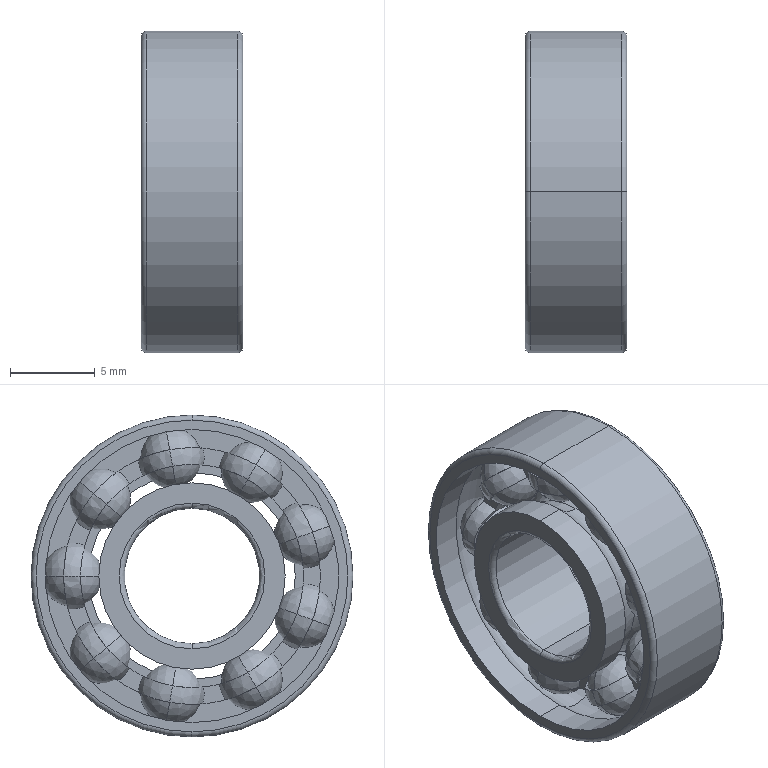Part | NX | features BREP 3 | 3 solids | 130 faces | box 6 x 19 x 19 mm | volume 760.399 mm3 | sphere 72 | plane 24 | cylinder 20 | torus 14 | commonest cylinder face diameters 17.3 x6 11 x4 8 x2 12.188 x2 13.16 x2 15.14 x2